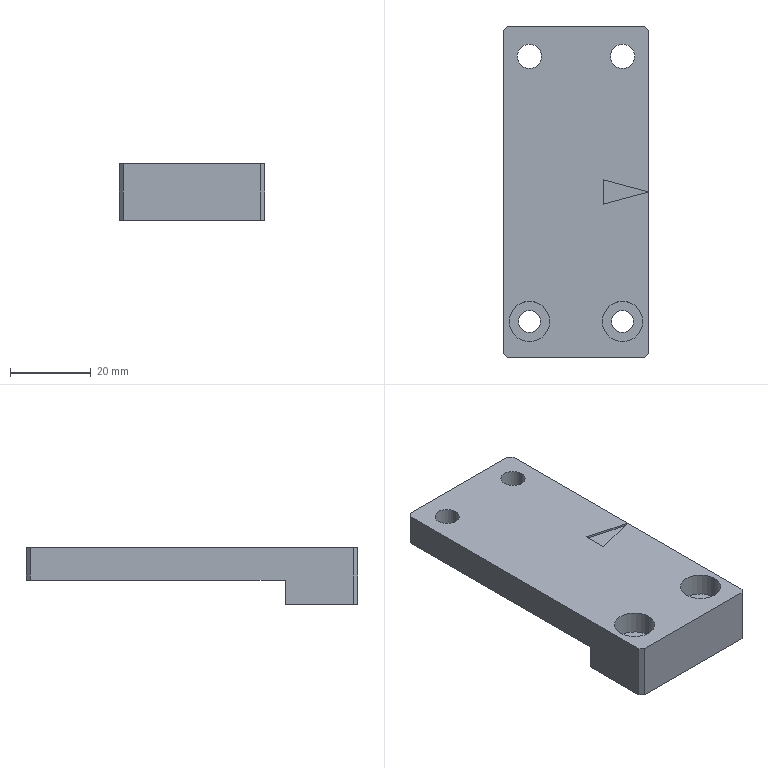Part | SolidWorks | features ICE 2, Chamfer 1, Extrusion 1, HoleWzd 1 | 1 solid | 30 faces | box 36 x 82 x 14 mm | volume 25723 mm3 | plane 18 | cylinder 12 | commonest cylinder face diameters 5.5 x4 6 x4 10 x4
STEP:
#1=CARTESIAN_POINT('',(8.5,74.5,-8.));
#2=VERTEX_POINT('',#1);
#3=CARTESIAN_POINT('',(14.5,74.5,-8.));
#4=VERTEX_POINT('',#3);
#5=CARTESIAN_POINT('',(11.5,74.5,-8.));
#6=DIRECTION('',(0.,0.,1.));
#7=DIRECTION('',(0.,-1.,0.));
#8=AXIS2_PLACEMENT_3D('',#5,#6,#7);
#9=CIRCLE('',#8,3.);
#10=EDGE_CURVE('',#2,#4,#9,.T.);
#11=ORIENTED_EDGE('',*,*,#10,.F.);
#12=CARTESIAN_POINT('',(8.5,74.5,0.));
#13=VERTEX_POINT('',#12);
#14=CARTESIAN_POINT('',(8.5,74.5,-14.));
#15=DIRECTION('',(0.,0.,1.));
#16=VECTOR('',#15,1000.);
#17=LINE('',#14,#16);
#18=EDGE_CURVE('',#2,#13,#17,.T.);
#19=ORIENTED_EDGE('',*,*,#18,.T.);
#20=CARTESIAN_POINT('',(14.5,74.5,0.));
#21=VERTEX_POINT('',#20);
#22=CARTESIAN_POINT('',(11.5,74.5,0.));
#23=DIRECTION('',(0.,0.,1.));
#24=DIRECTION('',(-1.,0.,0.));
#25=AXIS2_PLACEMENT_3D('',#22,#23,#24);
#26=CIRCLE('',#25,3.);
#27=EDGE_CURVE('',#13,#21,#26,.T.);
#28=ORIENTED_EDGE('',*,*,#27,.T.);
#29=CARTESIAN_POINT('',(14.5,74.5,-14.));
#30=DIRECTION('',(0.,0.,1.));
#31=VECTOR('',#30,1000.);
#32=LINE('',#29,#31);
#33=EDGE_CURVE('',#4,#21,#32,.T.);
#34=ORIENTED_EDGE('',*,*,#33,.F.);
#35=EDGE_LOOP('',(#11,#19,#28,#34));
#36=FACE_OUTER_BOUND('',#35,.T.);
#37=CARTESIAN_POINT('',(11.5,74.5,-14.));
#38=DIRECTION('',(0.,0.,1.));
#39=DIRECTION('',(1.,0.,0.));
#40=AXIS2_PLACEMENT_3D('',#37,#38,#39);
#41=CYLINDRICAL_SURFACE('',#40,3.);
#42=ADVANCED_FACE('',(#36),#41,.F.);
#43=CARTESIAN_POINT('',(-14.5,74.5,-8.));
#44=VERTEX_POINT('',#43);
#45=CARTESIAN_POINT('',(-8.5,74.5,-8.));
#46=VERTEX_POINT('',#45);
#47=CARTESIAN_POINT('',(-11.5,74.5,-8.));
#48=DIRECTION('',(0.,0.,1.));
#49=DIRECTION('',(0.,-1.,0.));
#50=AXIS2_PLACEMENT_3D('',#47,#48,#49);
#51=CIRCLE('',#50,3.);
#52=EDGE_CURVE('',#44,#46,#51,.T.);
#53=ORIENTED_EDGE('',*,*,#52,.F.);
#54=CARTESIAN_POINT('',(-14.5,74.5,0.));
#55=VERTEX_POINT('',#54);
#56=CARTESIAN_POINT('',(-14.5,74.5,-14.));
#57=DIRECTION('',(0.,0.,1.));
#58=VECTOR('',#57,1000.);
#59=LINE('',#56,#58);
#60=EDGE_CURVE('',#44,#55,#59,.T.);
#61=ORIENTED_EDGE('',*,*,#60,.T.);
#62=CARTESIAN_POINT('',(-8.5,74.5,0.));
#63=VERTEX_POINT('',#62);
#64=CARTESIAN_POINT('',(-11.5,74.5,0.));
#65=DIRECTION('',(0.,0.,1.));
#66=DIRECTION('',(1.,0.,0.));
#67=AXIS2_PLACEMENT_3D('',#64,#65,#66);
#68=CIRCLE('',#67,3.);
#69=EDGE_CURVE('',#55,#63,#68,.T.);
#70=ORIENTED_EDGE('',*,*,#69,.T.);
#71=CARTESIAN_POINT('',(-8.5,74.5,-14.));
#72=DIRECTION('',(0.,0.,1.));
#73=VECTOR('',#72,1000.);
#74=LINE('',#71,#73);
#75=EDGE_CURVE('',#46,#63,#74,.T.);
#76=ORIENTED_EDGE('',*,*,#75,.F.);
#77=EDGE_LOOP('',(#53,#61,#70,#76));
#78=FACE_OUTER_BOUND('',#77,.T.);
#79=CARTESIAN_POINT('',(-11.5,74.5,-14.));
#80=DIRECTION('',(0.,0.,1.));
#81=DIRECTION('',(1.,0.,0.));
#82=AXIS2_PLACEMENT_3D('',#79,#80,#81);
#83=CYLINDRICAL_SURFACE('',#82,3.);
#84=ADVANCED_FACE('',(#78),#83,.F.);
#85=CARTESIAN_POINT('',(6.5,9.,-5.7));
#86=VERTEX_POINT('',#85);
#87=CARTESIAN_POINT('',(16.5,9.,-5.7));
#88=VERTEX_POINT('',#87);
#89=CARTESIAN_POINT('',(11.5,9.,-5.7));
#90=DIRECTION('',(0.,0.,1.));
#91=DIRECTION('',(1.,0.,0.));
#92=AXIS2_PLACEMENT_3D('',#89,#90,#91);
#93=CIRCLE('',#92,5.);
#94=EDGE_CURVE('',#86,#88,#93,.T.);
#95=ORIENTED_EDGE('',*,*,#94,.F.);
#96=CARTESIAN_POINT('',(6.5,9.,0.));
#97=VERTEX_POINT('',#96);
#98=CARTESIAN_POINT('',(6.5,9.,0.));
#99=DIRECTION('',(0.,0.,1.));
#100=VECTOR('',#99,1000.);
#101=LINE('',#98,#100);
#102=EDGE_CURVE('',#86,#97,#101,.T.);
#103=ORIENTED_EDGE('',*,*,#102,.T.);
#104=CARTESIAN_POINT('',(16.5,9.,0.));
#105=VERTEX_POINT('',#104);
#106=CARTESIAN_POINT('',(11.5,9.,0.));
#107=DIRECTION('',(0.,0.,1.));
#108=DIRECTION('',(1.,0.,0.));
#109=AXIS2_PLACEMENT_3D('',#106,#107,#108);
#110=CIRCLE('',#109,5.);
#111=EDGE_CURVE('',#97,#105,#110,.T.);
#112=ORIENTED_EDGE('',*,*,#111,.T.);
#113=CARTESIAN_POINT('',(16.5,9.,0.));
#114=DIRECTION('',(0.,0.,1.));
#115=VECTOR('',#114,1000.);
#116=LINE('',#113,#115);
#117=EDGE_CURVE('',#88,#105,#116,.T.);
#118=ORIENTED_EDGE('',*,*,#117,.F.);
#119=EDGE_LOOP('',(#95,#103,#112,#118));
#120=FACE_OUTER_BOUND('',#119,.T.);
#121=CARTESIAN_POINT('',(11.5,9.,0.));
#122=DIRECTION('',(0.,0.,1.));
#123=DIRECTION('',(1.,0.,0.));
#124=AXIS2_PLACEMENT_3D('',#121,#122,#123);
#125=CYLINDRICAL_SURFACE('',#124,5.);
#126=ADVANCED_FACE('',(#120),#125,.F.);
#127=CARTESIAN_POINT('',(8.75,9.,-14.));
#128=VERTEX_POINT('',#127);
#129=CARTESIAN_POINT('',(14.25,9.,-14.));
#130=VERTEX_POINT('',#129);
#131=CARTESIAN_POINT('',(11.5,9.,-14.));
#132=DIRECTION('',(0.,0.,1.));
#133=DIRECTION('',(1.,0.,0.));
#134=AXIS2_PLACEMENT_3D('',#131,#132,#133);
#135=CIRCLE('',#134,2.75);
#136=EDGE_CURVE('',#128,#130,#135,.T.);
#137=ORIENTED_EDGE('',*,*,#136,.F.);
#138=CARTESIAN_POINT('',(8.75,9.,-5.7));
#139=VERTEX_POINT('',#138);
#140=CARTESIAN_POINT('',(8.75,9.,0.));
#141=DIRECTION('',(0.,0.,1.));
#142=VECTOR('',#141,1000.);
#143=LINE('',#140,#142);
#144=EDGE_CURVE('',#128,#139,#143,.T.);
#145=ORIENTED_EDGE('',*,*,#144,.T.);
#146=CARTESIAN_POINT('',(14.25,9.,-5.7));
#147=VERTEX_POINT('',#146);
#148=CARTESIAN_POINT('',(11.5,9.,-5.7));
#149=DIRECTION('',(0.,0.,1.));
#150=DIRECTION('',(1.,0.,0.));
#151=AXIS2_PLACEMENT_3D('',#148,#149,#150);
#152=CIRCLE('',#151,2.75);
#153=EDGE_CURVE('',#139,#147,#152,.T.);
#154=ORIENTED_EDGE('',*,*,#153,.T.);
#155=CARTESIAN_POINT('',(14.25,9.,0.));
#156=DIRECTION('',(0.,0.,1.));
#157=VECTOR('',#156,1000.);
#158=LINE('',#155,#157);
#159=EDGE_CURVE('',#130,#147,#158,.T.);
#160=ORIENTED_EDGE('',*,*,#159,.F.);
#161=EDGE_LOOP('',(#137,#145,#154,#160));
#162=FACE_OUTER_BOUND('',#161,.T.);
#163=CARTESIAN_POINT('',(11.5,9.,0.));
#164=DIRECTION('',(0.,0.,1.));
#165=DIRECTION('',(1.,0.,0.));
#166=AXIS2_PLACEMENT_3D('',#163,#164,#165);
#167=CYLINDRICAL_SURFACE('',#166,2.75);
#168=ADVANCED_FACE('',(#162),#167,.F.);
#169=CARTESIAN_POINT('',(-16.5,9.,-5.7));
#170=VERTEX_POINT('',#169);
#171=CARTESIAN_POINT('',(-6.5,9.,-5.7));
#172=VERTEX_POINT('',#171);
#173=CARTESIAN_POINT('',(-11.5,9.,-5.7));
#174=DIRECTION('',(0.,0.,1.));
#175=DIRECTION('',(1.,0.,0.));
#176=AXIS2_PLACEMENT_3D('',#173,#174,#175);
#177=CIRCLE('',#176,5.);
#178=EDGE_CURVE('',#170,#172,#177,.T.);
#179=ORIENTED_EDGE('',*,*,#178,.F.);
#180=CARTESIAN_POINT('',(-16.5,9.,0.));
#181=VERTEX_POINT('',#180);
#182=CARTESIAN_POINT('',(-16.5,9.,0.));
#183=DIRECTION('',(0.,0.,1.));
#184=VECTOR('',#183,1000.);
#185=LINE('',#182,#184);
#186=EDGE_CURVE('',#170,#181,#185,.T.);
#187=ORIENTED_EDGE('',*,*,#186,.T.);
#188=CARTESIAN_POINT('',(-6.5,9.,0.));
#189=VERTEX_POINT('',#188);
#190=CARTESIAN_POINT('',(-11.5,9.,0.));
#191=DIRECTION('',(0.,0.,1.));
#192=DIRECTION('',(1.,0.,0.));
#193=AXIS2_PLACEMENT_3D('',#190,#191,#192);
#194=CIRCLE('',#193,5.);
#195=EDGE_CURVE('',#181,#189,#194,.T.);
#196=ORIENTED_EDGE('',*,*,#195,.T.);
#197=CARTESIAN_POINT('',(-6.5,9.,0.));
#198=DIRECTION('',(0.,0.,1.));
#199=VECTOR('',#198,1000.);
#200=LINE('',#197,#199);
#201=EDGE_CURVE('',#172,#189,#200,.T.);
#202=ORIENTED_EDGE('',*,*,#201,.F.);
#203=EDGE_LOOP('',(#179,#187,#196,#202));
#204=FACE_OUTER_BOUND('',#203,.T.);
#205=CARTESIAN_POINT('',(-11.5,9.,0.));
#206=DIRECTION('',(0.,0.,1.));
#207=DIRECTION('',(1.,0.,0.));
#208=AXIS2_PLACEMENT_3D('',#205,#206,#207);
#209=CYLINDRICAL_SURFACE('',#208,5.);
#210=ADVANCED_FACE('',(#204),#209,.F.);
#211=CARTESIAN_POINT('',(-14.25,9.,-14.));
#212=VERTEX_POINT('',#211);
#213=CARTESIAN_POINT('',(-8.75,9.,-14.));
#214=VERTEX_POINT('',#213);
#215=CARTESIAN_POINT('',(-11.5,9.,-14.));
#216=DIRECTION('',(0.,0.,1.));
#217=DIRECTION('',(1.,0.,0.));
#218=AXIS2_PLACEMENT_3D('',#215,#216,#217);
#219=CIRCLE('',#218,2.75);
#220=EDGE_CURVE('',#212,#214,#219,.T.);
#221=ORIENTED_EDGE('',*,*,#220,.F.);
#222=CARTESIAN_POINT('',(-14.25,9.,-5.7));
#223=VERTEX_POINT('',#222);
#224=CARTESIAN_POINT('',(-14.25,9.,0.));
#225=DIRECTION('',(0.,0.,1.));
#226=VECTOR('',#225,1000.);
#227=LINE('',#224,#226);
#228=EDGE_CURVE('',#212,#223,#227,.T.);
#229=ORIENTED_EDGE('',*,*,#228,.T.);
#230=CARTESIAN_POINT('',(-8.75,9.,-5.7));
#231=VERTEX_POINT('',#230);
#232=CARTESIAN_POINT('',(-11.5,9.,-5.7));
#233=DIRECTION('',(0.,0.,1.));
#234=DIRECTION('',(1.,0.,0.));
#235=AXIS2_PLACEMENT_3D('',#232,#233,#234);
#236=CIRCLE('',#235,2.75);
#237=EDGE_CURVE('',#223,#231,#236,.T.);
#238=ORIENTED_EDGE('',*,*,#237,.T.);
#239=CARTESIAN_POINT('',(-8.75,9.,0.));
#240=DIRECTION('',(0.,0.,1.));
#241=VECTOR('',#240,1000.);
#242=LINE('',#239,#241);
#243=EDGE_CURVE('',#214,#231,#242,.T.);
#244=ORIENTED_EDGE('',*,*,#243,.F.);
#245=EDGE_LOOP('',(#221,#229,#238,#244));
#246=FACE_OUTER_BOUND('',#245,.T.);
#247=CARTESIAN_POINT('',(-11.5,9.,0.));
#248=DIRECTION('',(0.,0.,1.));
#249=DIRECTION('',(1.,0.,0.));
#250=AXIS2_PLACEMENT_3D('',#247,#248,#249);
#251=CYLINDRICAL_SURFACE('',#250,2.75);
#252=ADVANCED_FACE('',(#246),#251,.F.);
#253=CARTESIAN_POINT('',(11.5,9.,-14.));
#254=DIRECTION('',(0.,0.,1.));
#255=DIRECTION('',(1.,0.,0.));
#256=AXIS2_PLACEMENT_3D('',#253,#254,#255);
#257=CIRCLE('',#256,2.75);
#258=EDGE_CURVE('',#130,#128,#257,.T.);
#259=ORIENTED_EDGE('',*,*,#258,.T.);
#260=ORIENTED_EDGE('',*,*,#136,.T.);
#261=EDGE_LOOP('',(#259,#260));
#262=FACE_BOUND('',#261,.T.);
#263=CARTESIAN_POINT('',(-11.5,9.,-14.));
#264=DIRECTION('',(0.,0.,1.));
#265=DIRECTION('',(1.,0.,0.));
#266=AXIS2_PLACEMENT_3D('',#263,#264,#265);
#267=CIRCLE('',#266,2.75);
#268=EDGE_CURVE('',#214,#212,#267,.T.);
#269=ORIENTED_EDGE('',*,*,#268,.T.);
#270=ORIENTED_EDGE('',*,*,#220,.T.);
#271=EDGE_LOOP('',(#269,#270));
#272=FACE_BOUND('',#271,.T.);
#273=CARTESIAN_POINT('',(17.,0.,-14.));
#274=VERTEX_POINT('',#273);
#275=CARTESIAN_POINT('',(-17.,0.,-14.));
#276=VERTEX_POINT('',#275);
#277=CARTESIAN_POINT('',(18.,0.,-14.));
#278=DIRECTION('',(-1.,0.,0.));
#279=VECTOR('',#278,1000.);
#280=LINE('',#277,#279);
#281=EDGE_CURVE('',#274,#276,#280,.T.);
#282=ORIENTED_EDGE('',*,*,#281,.T.);
#283=CARTESIAN_POINT('',(-18.,1.,-14.));
#284=VERTEX_POINT('',#283);
#285=CARTESIAN_POINT('',(-17.,0.,-14.));
#286=DIRECTION('',(-0.7071,0.7071,0.));
#287=VECTOR('',#286,1000.);
#288=LINE('',#285,#287);
#289=EDGE_CURVE('',#276,#284,#288,.T.);
#290=ORIENTED_EDGE('',*,*,#289,.T.);
#291=CARTESIAN_POINT('',(-18.,18.,-14.));
#292=VERTEX_POINT('',#291);
#293=CARTESIAN_POINT('',(-18.,18.,-14.));
#294=DIRECTION('',(0.,1.,0.));
#295=VECTOR('',#294,1000.);
#296=LINE('',#293,#295);
#297=EDGE_CURVE('',#284,#292,#296,.T.);
#298=ORIENTED_EDGE('',*,*,#297,.T.);
#299=CARTESIAN_POINT('',(18.,18.,-14.));
#300=VERTEX_POINT('',#299);
#301=CARTESIAN_POINT('',(18.,18.,-14.));
#302=DIRECTION('',(-1.,0.,0.));
#303=VECTOR('',#302,1000.);
#304=LINE('',#301,#303);
#305=EDGE_CURVE('',#300,#292,#304,.T.);
#306=ORIENTED_EDGE('',*,*,#305,.F.);
#307=CARTESIAN_POINT('',(18.,1.,-14.));
#308=VERTEX_POINT('',#307);
#309=CARTESIAN_POINT('',(18.,18.,-14.));
#310=DIRECTION('',(0.,1.,0.));
#311=VECTOR('',#310,1000.);
#312=LINE('',#309,#311);
#313=EDGE_CURVE('',#308,#300,#312,.T.);
#314=ORIENTED_EDGE('',*,*,#313,.F.);
#315=CARTESIAN_POINT('',(18.,1.,-14.));
#316=DIRECTION('',(-0.7071,-0.7071,0.));
#317=VECTOR('',#316,1000.);
#318=LINE('',#315,#317);
#319=EDGE_CURVE('',#308,#274,#318,.T.);
#320=ORIENTED_EDGE('',*,*,#319,.T.);
#321=EDGE_LOOP('',(#282,#290,#298,#306,#314,#320));
#322=FACE_OUTER_BOUND('',#321,.T.);
#323=CARTESIAN_POINT('',(18.,18.,-14.));
#324=DIRECTION('',(0.,0.,1.));
#325=DIRECTION('',(0.,-1.,0.));
#326=AXIS2_PLACEMENT_3D('',#323,#324,#325);
#327=PLANE('',#326);
#328=ADVANCED_FACE('',(#262,#272,#322),#327,.F.);
#329=CARTESIAN_POINT('',(-18.,18.,-8.));
#330=VERTEX_POINT('',#329);
#331=CARTESIAN_POINT('',(-18.,18.,-8.));
#332=DIRECTION('',(0.,0.,1.));
#333=VECTOR('',#332,1000.);
#334=LINE('',#331,#333);
#335=EDGE_CURVE('',#292,#330,#334,.T.);
#336=ORIENTED_EDGE('',*,*,#335,.T.);
#337=CARTESIAN_POINT('',(18.,18.,-8.));
#338=VERTEX_POINT('',#337);
#339=CARTESIAN_POINT('',(18.,18.,-8.));
#340=DIRECTION('',(-1.,0.,0.));
#341=VECTOR('',#340,1000.);
#342=LINE('',#339,#341);
#343=EDGE_CURVE('',#338,#330,#342,.T.);
#344=ORIENTED_EDGE('',*,*,#343,.F.);
#345=CARTESIAN_POINT('',(18.,18.,-8.));
#346=DIRECTION('',(0.,0.,1.));
#347=VECTOR('',#346,1000.);
#348=LINE('',#345,#347);
#349=EDGE_CURVE('',#300,#338,#348,.T.);
#350=ORIENTED_EDGE('',*,*,#349,.F.);
#351=ORIENTED_EDGE('',*,*,#305,.T.);
#352=EDGE_LOOP('',(#336,#344,#350,#351));
#353=FACE_OUTER_BOUND('',#352,.T.);
#354=CARTESIAN_POINT('',(18.,18.,-8.));
#355=DIRECTION('',(0.,-1.,0.));
#356=DIRECTION('',(0.,0.,-1.));
#357=AXIS2_PLACEMENT_3D('',#354,#355,#356);
#358=PLANE('',#357);
#359=ADVANCED_FACE('',(#353),#358,.F.);
#360=CARTESIAN_POINT('',(11.5,74.5,-8.));
#361=DIRECTION('',(0.,0.,1.));
#362=DIRECTION('',(0.,-1.,0.));
#363=AXIS2_PLACEMENT_3D('',#360,#361,#362);
#364=CIRCLE('',#363,3.);
#365=EDGE_CURVE('',#4,#2,#364,.T.);
#366=ORIENTED_EDGE('',*,*,#365,.T.);
#367=ORIENTED_EDGE('',*,*,#10,.T.);
#368=EDGE_LOOP('',(#366,#367));
#369=FACE_BOUND('',#368,.T.);
#370=CARTESIAN_POINT('',(-11.5,74.5,-8.));
#371=DIRECTION('',(0.,0.,1.));
#372=DIRECTION('',(0.,-1.,0.));
#373=AXIS2_PLACEMENT_3D('',#370,#371,#372);
#374=CIRCLE('',#373,3.);
#375=EDGE_CURVE('',#46,#44,#374,.T.);
#376=ORIENTED_EDGE('',*,*,#375,.T.);
#377=ORIENTED_EDGE('',*,*,#52,.T.);
#378=EDGE_LOOP('',(#376,#377));
#379=FACE_BOUND('',#378,.T.);
#380=CARTESIAN_POINT('',(17.,82.,-8.));
#381=VERTEX_POINT('',#380);
#382=CARTESIAN_POINT('',(-17.,82.,-8.));
#383=VERTEX_POINT('',#382);
#384=CARTESIAN_POINT('',(18.,82.,-8.));
#385=DIRECTION('',(-1.,0.,0.));
#386=VECTOR('',#385,1000.);
#387=LINE('',#384,#386);
#388=EDGE_CURVE('',#381,#383,#387,.T.);
#389=ORIENTED_EDGE('',*,*,#388,.F.);
#390=CARTESIAN_POINT('',(18.,81.,-8.));
#391=VERTEX_POINT('',#390);
#392=CARTESIAN_POINT('',(18.,81.,-8.));
#393=DIRECTION('',(0.7071,-0.7071,0.));
#394=VECTOR('',#393,1000.);
#395=LINE('',#392,#394);
#396=EDGE_CURVE('',#381,#391,#395,.T.);
#397=ORIENTED_EDGE('',*,*,#396,.T.);
#398=CARTESIAN_POINT('',(18.,82.,-8.));
#399=DIRECTION('',(0.,1.,0.));
#400=VECTOR('',#399,1000.);
#401=LINE('',#398,#400);
#402=EDGE_CURVE('',#338,#391,#401,.T.);
#403=ORIENTED_EDGE('',*,*,#402,.F.);
#404=ORIENTED_EDGE('',*,*,#343,.T.);
#405=CARTESIAN_POINT('',(-18.,81.,-8.));
#406=VERTEX_POINT('',#405);
#407=CARTESIAN_POINT('',(-18.,82.,-8.));
#408=DIRECTION('',(0.,1.,0.));
#409=VECTOR('',#408,1000.);
#410=LINE('',#407,#409);
#411=EDGE_CURVE('',#330,#406,#410,.T.);
#412=ORIENTED_EDGE('',*,*,#411,.T.);
#413=CARTESIAN_POINT('',(-17.,82.,-8.));
#414=DIRECTION('',(0.7071,0.7071,0.));
#415=VECTOR('',#414,1000.);
#416=LINE('',#413,#415);
#417=EDGE_CURVE('',#406,#383,#416,.T.);
#418=ORIENTED_EDGE('',*,*,#417,.T.);
#419=EDGE_LOOP('',(#389,#397,#403,#404,#412,#418));
#420=FACE_OUTER_BOUND('',#419,.T.);
#421=CARTESIAN_POINT('',(18.,82.,-8.));
#422=DIRECTION('',(0.,0.,1.));
#423=DIRECTION('',(0.,-1.,0.));
#424=AXIS2_PLACEMENT_3D('',#421,#422,#423);
#425=PLANE('',#424);
#426=ADVANCED_FACE('',(#369,#379,#420),#425,.F.);
#427=CARTESIAN_POINT('',(17.,82.,0.));
#428=VERTEX_POINT('',#427);
#429=CARTESIAN_POINT('',(-17.,82.,0.));
#430=VERTEX_POINT('',#429);
#431=CARTESIAN_POINT('',(18.,82.,0.));
#432=DIRECTION('',(-1.,0.,0.));
#433=VECTOR('',#432,1000.);
#434=LINE('',#431,#433);
#435=EDGE_CURVE('',#428,#430,#434,.T.);
#436=ORIENTED_EDGE('',*,*,#435,.F.);
#437=CARTESIAN_POINT('',(17.,82.,0.));
#438=DIRECTION('',(0.,0.,-1.));
#439=VECTOR('',#438,1000.);
#440=LINE('',#437,#439);
#441=EDGE_CURVE('',#428,#381,#440,.T.);
#442=ORIENTED_EDGE('',*,*,#441,.T.);
#443=ORIENTED_EDGE('',*,*,#388,.T.);
#444=CARTESIAN_POINT('',(-17.,82.,0.));
#445=DIRECTION('',(0.,0.,1.));
#446=VECTOR('',#445,1000.);
#447=LINE('',#444,#446);
#448=EDGE_CURVE('',#383,#430,#447,.T.);
#449=ORIENTED_EDGE('',*,*,#448,.T.);
#450=EDGE_LOOP('',(#436,#442,#443,#449));
#451=FACE_OUTER_BOUND('',#450,.T.);
#452=CARTESIAN_POINT('',(18.,82.,0.));
#453=DIRECTION('',(0.,-1.,0.));
#454=DIRECTION('',(0.,0.,-1.));
#455=AXIS2_PLACEMENT_3D('',#452,#453,#454);
#456=PLANE('',#455);
#457=ADVANCED_FACE('',(#451),#456,.F.);
#458=CARTESIAN_POINT('',(6.7,38.,0.));
#459=VERTEX_POINT('',#458);
#460=CARTESIAN_POINT('',(17.896,41.,0.));
#461=VERTEX_POINT('',#460);
#462=CARTESIAN_POINT('',(17.896,41.,0.));
#463=DIRECTION('',(0.9659,0.2588,0.));
#464=VECTOR('',#463,1000.);
#465=LINE('',#462,#464);
#466=EDGE_CURVE('',#459,#461,#465,.T.);
#467=ORIENTED_EDGE('',*,*,#466,.F.);
#468=CARTESIAN_POINT('',(6.7,44.,0.));
#469=VERTEX_POINT('',#468);
#470=CARTESIAN_POINT('',(6.7,38.,0.));
#471=DIRECTION('',(0.,-1.,0.));
#472=VECTOR('',#471,1000.);
#473=LINE('',#470,#472);
#474=EDGE_CURVE('',#469,#459,#473,.T.);
#475=ORIENTED_EDGE('',*,*,#474,.F.);
#476=CARTESIAN_POINT('',(6.7,44.,0.));
#477=DIRECTION('',(-0.9659,0.2588,0.));
#478=VECTOR('',#477,1000.);
#479=LINE('',#476,#478);
#480=EDGE_CURVE('',#461,#469,#479,.T.);
#481=ORIENTED_EDGE('',*,*,#480,.F.);
#482=EDGE_LOOP('',(#467,#475,#481));
#483=FACE_BOUND('',#482,.T.);
#484=CARTESIAN_POINT('',(11.5,74.5,0.));
#485=DIRECTION('',(0.,0.,1.));
#486=DIRECTION('',(-1.,0.,0.));
#487=AXIS2_PLACEMENT_3D('',#484,#485,#486);
#488=CIRCLE('',#487,3.);
#489=EDGE_CURVE('',#21,#13,#488,.T.);
#490=ORIENTED_EDGE('',*,*,#489,.F.);
#491=ORIENTED_EDGE('',*,*,#27,.F.);
#492=EDGE_LOOP('',(#490,#491));
#493=FACE_BOUND('',#492,.T.);
#494=CARTESIAN_POINT('',(-11.5,74.5,0.));
#495=DIRECTION('',(0.,0.,1.));
#496=DIRECTION('',(1.,0.,0.));
#497=AXIS2_PLACEMENT_3D('',#494,#495,#496);
#498=CIRCLE('',#497,3.);
#499=EDGE_CURVE('',#63,#55,#498,.T.);
#500=ORIENTED_EDGE('',*,*,#499,.F.);
#501=ORIENTED_EDGE('',*,*,#69,.F.);
#502=EDGE_LOOP('',(#500,#501));
#503=FACE_BOUND('',#502,.T.);
#504=CARTESIAN_POINT('',(11.5,9.,0.));
#505=DIRECTION('',(0.,0.,1.));
#506=DIRECTION('',(1.,0.,0.));
#507=AXIS2_PLACEMENT_3D('',#504,#505,#506);
#508=CIRCLE('',#507,5.);
#509=EDGE_CURVE('',#105,#97,#508,.T.);
#510=ORIENTED_EDGE('',*,*,#509,.F.);
#511=ORIENTED_EDGE('',*,*,#111,.F.);
#512=EDGE_LOOP('',(#510,#511));
#513=FACE_BOUND('',#512,.T.);
#514=CARTESIAN_POINT('',(-11.5,9.,0.));
#515=DIRECTION('',(0.,0.,1.));
#516=DIRECTION('',(1.,0.,0.));
#517=AXIS2_PLACEMENT_3D('',#514,#515,#516);
#518=CIRCLE('',#517,5.);
#519=EDGE_CURVE('',#189,#181,#518,.T.);
#520=ORIENTED_EDGE('',*,*,#519,.F.);
#521=ORIENTED_EDGE('',*,*,#195,.F.);
#522=EDGE_LOOP('',(#520,#521));
#523=FACE_BOUND('',#522,.T.);
#524=CARTESIAN_POINT('',(-18.,81.,0.));
#525=VERTEX_POINT('',#524);
#526=CARTESIAN_POINT('',(-18.,1.,0.));
#527=VERTEX_POINT('',#526);
#528=CARTESIAN_POINT('',(-18.,0.,0.));
#529=DIRECTION('',(0.,-1.,0.));
#530=VECTOR('',#529,1000.);
#531=LINE('',#528,#530);
#532=EDGE_CURVE('',#525,#527,#531,.T.);
#533=ORIENTED_EDGE('',*,*,#532,.T.);
#534=CARTESIAN_POINT('',(-17.,0.,0.));
#535=VERTEX_POINT('',#534);
#536=CARTESIAN_POINT('',(-17.,0.,0.));
#537=DIRECTION('',(0.7071,-0.7071,0.));
#538=VECTOR('',#537,1000.);
#539=LINE('',#536,#538);
#540=EDGE_CURVE('',#527,#535,#539,.T.);
#541=ORIENTED_EDGE('',*,*,#540,.T.);
#542=CARTESIAN_POINT('',(17.,0.,0.));
#543=VERTEX_POINT('',#542);
#544=CARTESIAN_POINT('',(18.,0.,0.));
#545=DIRECTION('',(-1.,0.,0.));
#546=VECTOR('',#545,1000.);
#547=LINE('',#544,#546);
#548=EDGE_CURVE('',#543,#535,#547,.T.);
#549=ORIENTED_EDGE('',*,*,#548,.F.);
#550=CARTESIAN_POINT('',(18.,1.,0.));
#551=VERTEX_POINT('',#550);
#552=CARTESIAN_POINT('',(18.,1.,0.));
#553=DIRECTION('',(0.7071,0.7071,0.));
#554=VECTOR('',#553,1000.);
#555=LINE('',#552,#554);
#556=EDGE_CURVE('',#543,#551,#555,.T.);
#557=ORIENTED_EDGE('',*,*,#556,.T.);
#558=CARTESIAN_POINT('',(18.,81.,0.));
#559=VERTEX_POINT('',#558);
#560=CARTESIAN_POINT('',(18.,0.,0.));
#561=DIRECTION('',(0.,-1.,0.));
#562=VECTOR('',#561,1000.);
#563=LINE('',#560,#562);
#564=EDGE_CURVE('',#559,#551,#563,.T.);
#565=ORIENTED_EDGE('',*,*,#564,.F.);
#566=CARTESIAN_POINT('',(18.,81.,0.));
#567=DIRECTION('',(-0.7071,0.7071,0.));
#568=VECTOR('',#567,1000.);
#569=LINE('',#566,#568);
#570=EDGE_CURVE('',#559,#428,#569,.T.);
#571=ORIENTED_EDGE('',*,*,#570,.T.);
#572=ORIENTED_EDGE('',*,*,#435,.T.);
#573=CARTESIAN_POINT('',(-17.,82.,0.));
#574=DIRECTION('',(-0.7071,-0.7071,0.));
#575=VECTOR('',#574,1000.);
#576=LINE('',#573,#575);
#577=EDGE_CURVE('',#430,#525,#576,.T.);
#578=ORIENTED_EDGE('',*,*,#577,.T.);
#579=EDGE_LOOP('',(#533,#541,#549,#557,#565,#571,#572,#578));
#580=FACE_OUTER_BOUND('',#579,.T.);
#581=CARTESIAN_POINT('',(18.,0.,0.));
#582=DIRECTION('',(0.,0.,-1.));
#583=DIRECTION('',(0.,1.,0.));
#584=AXIS2_PLACEMENT_3D('',#581,#582,#583);
#585=PLANE('',#584);
#586=ADVANCED_FACE('',(#483,#493,#503,#513,#523,#580),#585,.F.);
#587=ORIENTED_EDGE('',*,*,#548,.T.);
#588=CARTESIAN_POINT('',(-17.,0.,-14.));
#589=DIRECTION('',(0.,0.,-1.));
#590=VECTOR('',#589,1000.);
#591=LINE('',#588,#590);
#592=EDGE_CURVE('',#535,#276,#591,.T.);
#593=ORIENTED_EDGE('',*,*,#592,.T.);
#594=ORIENTED_EDGE('',*,*,#281,.F.);
#595=CARTESIAN_POINT('',(17.,0.,-14.));
#596=DIRECTION('',(0.,0.,1.));
#597=VECTOR('',#596,1000.);
#598=LINE('',#595,#597);
#599=EDGE_CURVE('',#274,#543,#598,.T.);
#600=ORIENTED_EDGE('',*,*,#599,.T.);
#601=EDGE_LOOP('',(#587,#593,#594,#600));
#602=FACE_OUTER_BOUND('',#601,.T.);
#603=CARTESIAN_POINT('',(18.,0.,-14.));
#604=DIRECTION('',(0.,1.,0.));
#605=DIRECTION('',(0.,0.,1.));
#606=AXIS2_PLACEMENT_3D('',#603,#604,#605);
#607=PLANE('',#606);
#608=ADVANCED_FACE('',(#602),#607,.F.);
#609=ORIENTED_EDGE('',*,*,#564,.T.);
#610=CARTESIAN_POINT('',(18.,1.,-14.));
#611=DIRECTION('',(0.,0.,-1.));
#612=VECTOR('',#611,1000.);
#613=LINE('',#610,#612);
#614=EDGE_CURVE('',#551,#308,#613,.T.);
#615=ORIENTED_EDGE('',*,*,#614,.T.);
#616=ORIENTED_EDGE('',*,*,#313,.T.);
#617=ORIENTED_EDGE('',*,*,#349,.T.);
#618=ORIENTED_EDGE('',*,*,#402,.T.);
#619=CARTESIAN_POINT('',(18.,81.,-14.));
#620=DIRECTION('',(0.,0.,1.));
#621=VECTOR('',#620,1000.);
#622=LINE('',#619,#621);
#623=EDGE_CURVE('',#391,#559,#622,.T.);
#624=ORIENTED_EDGE('',*,*,#623,.T.);
#625=EDGE_LOOP('',(#609,#615,#616,#617,#618,#624));
#626=FACE_OUTER_BOUND('',#625,.T.);
#627=CARTESIAN_POINT('',(18.,0.,-14.));
#628=DIRECTION('',(-1.,0.,0.));
#629=DIRECTION('',(0.,0.,1.));
#630=AXIS2_PLACEMENT_3D('',#627,#628,#629);
#631=PLANE('',#630);
#632=ADVANCED_FACE('',(#626),#631,.F.);
#633=ORIENTED_EDGE('',*,*,#297,.F.);
#634=CARTESIAN_POINT('',(-18.,1.,0.));
#635=DIRECTION('',(0.,0.,1.));
#636=VECTOR('',#635,1000.);
#637=LINE('',#634,#636);
#638=EDGE_CURVE('',#284,#527,#637,.T.);
#639=ORIENTED_EDGE('',*,*,#638,.T.);
#640=ORIENTED_EDGE('',*,*,#532,.F.);
#641=CARTESIAN_POINT('',(-18.,81.,-8.));
#642=DIRECTION('',(0.,0.,-1.));
#643=VECTOR('',#642,1000.);
#644=LINE('',#641,#643);
#645=EDGE_CURVE('',#525,#406,#644,.T.);
#646=ORIENTED_EDGE('',*,*,#645,.T.);
#647=ORIENTED_EDGE('',*,*,#411,.F.);
#648=ORIENTED_EDGE('',*,*,#335,.F.);
#649=EDGE_LOOP('',(#633,#639,#640,#646,#647,#648));
#650=FACE_OUTER_BOUND('',#649,.T.);
#651=CARTESIAN_POINT('',(-18.,0.,-14.));
#652=DIRECTION('',(-1.,0.,0.));
#653=DIRECTION('',(0.,0.,1.));
#654=AXIS2_PLACEMENT_3D('',#651,#652,#653);
#655=PLANE('',#654);
#656=ADVANCED_FACE('',(#650),#655,.T.);
#657=ORIENTED_EDGE('',*,*,#228,.F.);
#658=ORIENTED_EDGE('',*,*,#268,.F.);
#659=ORIENTED_EDGE('',*,*,#243,.T.);
#660=CARTESIAN_POINT('',(-11.5,9.,-5.7));
#661=DIRECTION('',(0.,0.,1.));
#662=DIRECTION('',(1.,0.,0.));
#663=AXIS2_PLACEMENT_3D('',#660,#661,#662);
#664=CIRCLE('',#663,2.75);
#665=EDGE_CURVE('',#231,#223,#664,.T.);
#666=ORIENTED_EDGE('',*,*,#665,.T.);
#667=EDGE_LOOP('',(#657,#658,#659,#666));
#668=FACE_OUTER_BOUND('',#667,.T.);
#669=CARTESIAN_POINT('',(-11.5,9.,0.));
#670=DIRECTION('',(0.,0.,1.));
#671=DIRECTION('',(1.,0.,0.));
#672=AXIS2_PLACEMENT_3D('',#669,#670,#671);
#673=CYLINDRICAL_SURFACE('',#672,2.75);
#674=ADVANCED_FACE('',(#668),#673,.F.);
#675=ORIENTED_EDGE('',*,*,#665,.F.);
#676=ORIENTED_EDGE('',*,*,#237,.F.);
#677=EDGE_LOOP('',(#675,#676));
#678=FACE_BOUND('',#677,.T.);
#679=CARTESIAN_POINT('',(-11.5,9.,-5.7));
#680=DIRECTION('',(0.,0.,1.));
#681=DIRECTION('',(1.,0.,0.));
#682=AXIS2_PLACEMENT_3D('',#679,#680,#681);
#683=CIRCLE('',#682,5.);
#684=EDGE_CURVE('',#172,#170,#683,.T.);
#685=ORIENTED_EDGE('',*,*,#684,.T.);
#686=ORIENTED_EDGE('',*,*,#178,.T.);
#687=EDGE_LOOP('',(#685,#686));
#688=FACE_OUTER_BOUND('',#687,.T.);
#689=CARTESIAN_POINT('',(-8.75,9.,-5.7));
#690=DIRECTION('',(0.,0.,-1.));
#691=DIRECTION('',(-1.,0.,0.));
#692=AXIS2_PLACEMENT_3D('',#689,#690,#691);
#693=PLANE('',#692);
#694=ADVANCED_FACE('',(#678,#688),#693,.F.);
#695=ORIENTED_EDGE('',*,*,#186,.F.);
#696=ORIENTED_EDGE('',*,*,#684,.F.);
#697=ORIENTED_EDGE('',*,*,#201,.T.);
#698=ORIENTED_EDGE('',*,*,#519,.T.);
#699=EDGE_LOOP('',(#695,#696,#697,#698));
#700=FACE_OUTER_BOUND('',#699,.T.);
#701=CARTESIAN_POINT('',(-11.5,9.,0.));
#702=DIRECTION('',(0.,0.,1.));
#703=DIRECTION('',(1.,0.,0.));
#704=AXIS2_PLACEMENT_3D('',#701,#702,#703);
#705=CYLINDRICAL_SURFACE('',#704,5.);
#706=ADVANCED_FACE('',(#700),#705,.F.);
#707=ORIENTED_EDGE('',*,*,#144,.F.);
#708=ORIENTED_EDGE('',*,*,#258,.F.);
#709=ORIENTED_EDGE('',*,*,#159,.T.);
#710=CARTESIAN_POINT('',(11.5,9.,-5.7));
#711=DIRECTION('',(0.,0.,1.));
#712=DIRECTION('',(1.,0.,0.));
#713=AXIS2_PLACEMENT_3D('',#710,#711,#712);
#714=CIRCLE('',#713,2.75);
#715=EDGE_CURVE('',#147,#139,#714,.T.);
#716=ORIENTED_EDGE('',*,*,#715,.T.);
#717=EDGE_LOOP('',(#707,#708,#709,#716));
#718=FACE_OUTER_BOUND('',#717,.T.);
#719=CARTESIAN_POINT('',(11.5,9.,0.));
#720=DIRECTION('',(0.,0.,1.));
#721=DIRECTION('',(1.,0.,0.));
#722=AXIS2_PLACEMENT_3D('',#719,#720,#721);
#723=CYLINDRICAL_SURFACE('',#722,2.75);
#724=ADVANCED_FACE('',(#718),#723,.F.);
#725=ORIENTED_EDGE('',*,*,#715,.F.);
#726=ORIENTED_EDGE('',*,*,#153,.F.);
#727=EDGE_LOOP('',(#725,#726));
#728=FACE_BOUND('',#727,.T.);
#729=CARTESIAN_POINT('',(11.5,9.,-5.7));
#730=DIRECTION('',(0.,0.,1.));
#731=DIRECTION('',(1.,0.,0.));
#732=AXIS2_PLACEMENT_3D('',#729,#730,#731);
#733=CIRCLE('',#732,5.);
#734=EDGE_CURVE('',#88,#86,#733,.T.);
#735=ORIENTED_EDGE('',*,*,#734,.T.);
#736=ORIENTED_EDGE('',*,*,#94,.T.);
#737=EDGE_LOOP('',(#735,#736));
#738=FACE_OUTER_BOUND('',#737,.T.);
#739=CARTESIAN_POINT('',(14.25,9.,-5.7));
#740=DIRECTION('',(0.,0.,-1.));
#741=DIRECTION('',(-1.,0.,0.));
#742=AXIS2_PLACEMENT_3D('',#739,#740,#741);
#743=PLANE('',#742);
#744=ADVANCED_FACE('',(#728,#738),#743,.F.);
#745=ORIENTED_EDGE('',*,*,#102,.F.);
#746=ORIENTED_EDGE('',*,*,#734,.F.);
#747=ORIENTED_EDGE('',*,*,#117,.T.);
#748=ORIENTED_EDGE('',*,*,#509,.T.);
#749=EDGE_LOOP('',(#745,#746,#747,#748));
#750=FACE_OUTER_BOUND('',#749,.T.);
#751=CARTESIAN_POINT('',(11.5,9.,0.));
#752=DIRECTION('',(0.,0.,1.));
#753=DIRECTION('',(1.,0.,0.));
#754=AXIS2_PLACEMENT_3D('',#751,#752,#753);
#755=CYLINDRICAL_SURFACE('',#754,5.);
#756=ADVANCED_FACE('',(#750),#755,.F.);
#757=ORIENTED_EDGE('',*,*,#60,.F.);
#758=ORIENTED_EDGE('',*,*,#375,.F.);
#759=ORIENTED_EDGE('',*,*,#75,.T.);
#760=ORIENTED_EDGE('',*,*,#499,.T.);
#761=EDGE_LOOP('',(#757,#758,#759,#760));
#762=FACE_OUTER_BOUND('',#761,.T.);
#763=CARTESIAN_POINT('',(-11.5,74.5,-14.));
#764=DIRECTION('',(0.,0.,1.));
#765=DIRECTION('',(1.,0.,0.));
#766=AXIS2_PLACEMENT_3D('',#763,#764,#765);
#767=CYLINDRICAL_SURFACE('',#766,3.);
#768=ADVANCED_FACE('',(#762),#767,.F.);
#769=ORIENTED_EDGE('',*,*,#18,.F.);
#770=ORIENTED_EDGE('',*,*,#365,.F.);
#771=ORIENTED_EDGE('',*,*,#33,.T.);
#772=ORIENTED_EDGE('',*,*,#489,.T.);
#773=EDGE_LOOP('',(#769,#770,#771,#772));
#774=FACE_OUTER_BOUND('',#773,.T.);
#775=CARTESIAN_POINT('',(11.5,74.5,-14.));
#776=DIRECTION('',(0.,0.,1.));
#777=DIRECTION('',(1.,0.,0.));
#778=AXIS2_PLACEMENT_3D('',#775,#776,#777);
#779=CYLINDRICAL_SURFACE('',#778,3.);
#780=ADVANCED_FACE('',(#774),#779,.F.);
#781=ORIENTED_EDGE('',*,*,#540,.F.);
#782=ORIENTED_EDGE('',*,*,#638,.F.);
#783=ORIENTED_EDGE('',*,*,#289,.F.);
#784=ORIENTED_EDGE('',*,*,#592,.F.);
#785=EDGE_LOOP('',(#781,#782,#783,#784));
#786=FACE_OUTER_BOUND('',#785,.T.);
#787=CARTESIAN_POINT('',(-17.,0.,-14.));
#788=DIRECTION('',(-0.7071,-0.7071,0.));
#789=DIRECTION('',(0.7071,-0.7071,0.));
#790=AXIS2_PLACEMENT_3D('',#787,#788,#789);
#791=PLANE('',#790);
#792=ADVANCED_FACE('',(#786),#791,.T.);
#793=ORIENTED_EDGE('',*,*,#556,.F.);
#794=ORIENTED_EDGE('',*,*,#599,.F.);
#795=ORIENTED_EDGE('',*,*,#319,.F.);
#796=ORIENTED_EDGE('',*,*,#614,.F.);
#797=EDGE_LOOP('',(#793,#794,#795,#796));
#798=FACE_OUTER_BOUND('',#797,.T.);
#799=CARTESIAN_POINT('',(18.,1.,-14.));
#800=DIRECTION('',(-0.7071,0.7071,0.));
#801=DIRECTION('',(-0.7071,-0.7071,0.));
#802=AXIS2_PLACEMENT_3D('',#799,#800,#801);
#803=PLANE('',#802);
#804=ADVANCED_FACE('',(#798),#803,.F.);
#805=ORIENTED_EDGE('',*,*,#396,.F.);
#806=ORIENTED_EDGE('',*,*,#441,.F.);
#807=ORIENTED_EDGE('',*,*,#570,.F.);
#808=ORIENTED_EDGE('',*,*,#623,.F.);
#809=EDGE_LOOP('',(#805,#806,#807,#808));
#810=FACE_OUTER_BOUND('',#809,.T.);
#811=CARTESIAN_POINT('',(18.,81.,-14.));
#812=DIRECTION('',(-0.7071,-0.7071,0.));
#813=DIRECTION('',(0.7071,-0.7071,0.));
#814=AXIS2_PLACEMENT_3D('',#811,#812,#813);
#815=PLANE('',#814);
#816=ADVANCED_FACE('',(#810),#815,.F.);
#817=ORIENTED_EDGE('',*,*,#417,.F.);
#818=ORIENTED_EDGE('',*,*,#645,.F.);
#819=ORIENTED_EDGE('',*,*,#577,.F.);
#820=ORIENTED_EDGE('',*,*,#448,.F.);
#821=EDGE_LOOP('',(#817,#818,#819,#820));
#822=FACE_OUTER_BOUND('',#821,.T.);
#823=CARTESIAN_POINT('',(-17.,82.,0.));
#824=DIRECTION('',(-0.7071,0.7071,0.));
#825=DIRECTION('',(-0.7071,-0.7071,0.));
#826=AXIS2_PLACEMENT_3D('',#823,#824,#825);
#827=PLANE('',#826);
#828=ADVANCED_FACE('',(#822),#827,.T.);
#829=ORIENTED_EDGE('',*,*,#474,.T.);
#830=CARTESIAN_POINT('',(6.7,38.,-0.5));
#831=VERTEX_POINT('',#830);
#832=CARTESIAN_POINT('',(6.7,38.,-0.5));
#833=DIRECTION('',(0.,0.,1.));
#834=VECTOR('',#833,1000.);
#835=LINE('',#832,#834);
#836=EDGE_CURVE('',#831,#459,#835,.T.);
#837=ORIENTED_EDGE('',*,*,#836,.F.);
#838=CARTESIAN_POINT('',(6.7,44.,-0.5));
#839=VERTEX_POINT('',#838);
#840=CARTESIAN_POINT('',(6.7,38.,-0.5));
#841=DIRECTION('',(0.,-1.,0.));
#842=VECTOR('',#841,1000.);
#843=LINE('',#840,#842);
#844=EDGE_CURVE('',#839,#831,#843,.T.);
#845=ORIENTED_EDGE('',*,*,#844,.F.);
#846=CARTESIAN_POINT('',(6.7,44.,-0.5));
#847=DIRECTION('',(0.,0.,1.));
#848=VECTOR('',#847,1000.);
#849=LINE('',#846,#848);
#850=EDGE_CURVE('',#839,#469,#849,.T.);
#851=ORIENTED_EDGE('',*,*,#850,.T.);
#852=EDGE_LOOP('',(#829,#837,#845,#851));
#853=FACE_OUTER_BOUND('',#852,.T.);
#854=CARTESIAN_POINT('',(6.7,38.,-0.5));
#855=DIRECTION('',(-1.,0.,0.));
#856=DIRECTION('',(0.,-1.,0.));
#857=AXIS2_PLACEMENT_3D('',#854,#855,#856);
#858=PLANE('',#857);
#859=ADVANCED_FACE('',(#853),#858,.F.);
#860=ORIENTED_EDGE('',*,*,#480,.T.);
#861=ORIENTED_EDGE('',*,*,#850,.F.);
#862=CARTESIAN_POINT('',(17.896,41.,-0.5));
#863=VERTEX_POINT('',#862);
#864=CARTESIAN_POINT('',(6.7,44.,-0.5));
#865=DIRECTION('',(-0.9659,0.2588,0.));
#866=VECTOR('',#865,1000.);
#867=LINE('',#864,#866);
#868=EDGE_CURVE('',#863,#839,#867,.T.);
#869=ORIENTED_EDGE('',*,*,#868,.F.);
#870=CARTESIAN_POINT('',(17.896,41.,-0.5));
#871=DIRECTION('',(0.,0.,1.));
#872=VECTOR('',#871,1000.);
#873=LINE('',#870,#872);
#874=EDGE_CURVE('',#863,#461,#873,.T.);
#875=ORIENTED_EDGE('',*,*,#874,.T.);
#876=EDGE_LOOP('',(#860,#861,#869,#875));
#877=FACE_OUTER_BOUND('',#876,.T.);
#878=CARTESIAN_POINT('',(6.7,44.,-0.5));
#879=DIRECTION('',(0.2588,0.9659,0.));
#880=DIRECTION('',(-0.9659,0.2588,0.));
#881=AXIS2_PLACEMENT_3D('',#878,#879,#880);
#882=PLANE('',#881);
#883=ADVANCED_FACE('',(#877),#882,.F.);
#884=ORIENTED_EDGE('',*,*,#466,.T.);
#885=ORIENTED_EDGE('',*,*,#874,.F.);
#886=CARTESIAN_POINT('',(17.896,41.,-0.5));
#887=DIRECTION('',(0.9659,0.2588,0.));
#888=VECTOR('',#887,1000.);
#889=LINE('',#886,#888);
#890=EDGE_CURVE('',#831,#863,#889,.T.);
#891=ORIENTED_EDGE('',*,*,#890,.F.);
#892=ORIENTED_EDGE('',*,*,#836,.T.);
#893=EDGE_LOOP('',(#884,#885,#891,#892));
#894=FACE_OUTER_BOUND('',#893,.T.);
#895=CARTESIAN_POINT('',(17.896,41.,-0.5));
#896=DIRECTION('',(0.2588,-0.9659,0.));
#897=DIRECTION('',(0.9659,0.2588,0.));
#898=AXIS2_PLACEMENT_3D('',#895,#896,#897);
#899=PLANE('',#898);
#900=ADVANCED_FACE('',(#894),#899,.F.);
#901=ORIENTED_EDGE('',*,*,#844,.T.);
#902=ORIENTED_EDGE('',*,*,#890,.T.);
#903=ORIENTED_EDGE('',*,*,#868,.T.);
#904=EDGE_LOOP('',(#901,#902,#903));
#905=FACE_OUTER_BOUND('',#904,.T.);
#906=CARTESIAN_POINT('',(0.,0.,-0.5));
#907=DIRECTION('',(0.,0.,-1.));
#908=DIRECTION('',(-1.,0.,0.));
#909=AXIS2_PLACEMENT_3D('',#906,#907,#908);
#910=PLANE('',#909);
#911=ADVANCED_FACE('',(#905),#910,.F.);
#912=CLOSED_SHELL('',(#42,#84,#126,#168,#210,#252,#328,#359,#426,#457,#586,#608,#632,#656,#674,#694,#706,#724,#744,#756,#768,#780,#792,#804,#816,#828,#859,#883,#900,#911));
#913=MANIFOLD_SOLID_BREP('',#912);
#914=CARTESIAN_POINT('',(0.,0.,0.));
#915=DIRECTION('',(0.,0.,1.));
#916=DIRECTION('',(1.,0.,0.));
#917=AXIS2_PLACEMENT_3D('',#914,#915,#916);
#918=(LENGTH_UNIT()NAMED_UNIT(*)SI_UNIT(.MILLI.,.METRE.));
#919=UNCERTAINTY_MEASURE_WITH_UNIT(LENGTH_MEASURE(0.00001),#918,'','');
#920=(NAMED_UNIT(*)PLANE_ANGLE_UNIT()SI_UNIT($,.RADIAN.));
#921=(NAMED_UNIT(*)SI_UNIT($,.STERADIAN.)SOLID_ANGLE_UNIT());
#922=(GEOMETRIC_REPRESENTATION_CONTEXT(3)GLOBAL_UNCERTAINTY_ASSIGNED_CONTEXT((#919))GLOBAL_UNIT_ASSIGNED_CONTEXT((#918,#920,#921))REPRESENTATION_CONTEXT('',''));
#923=ADVANCED_BREP_SHAPE_REPRESENTATION('',(#913,#917),#922);